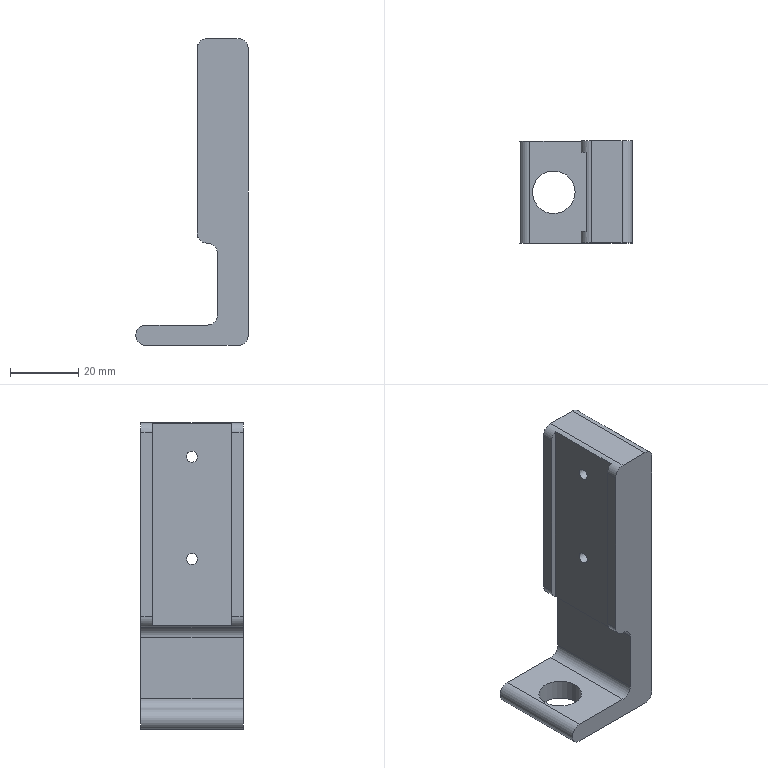Part | STEP file | SN10_008_004_SUPORTE | 1 solid | 22 faces | box 33 x 30 x 90 mm | volume 36222 mm3 | plane 12 | cylinder 10 | commonest cylinder face diameters 6 x7 3.242 x2 12.5 x1